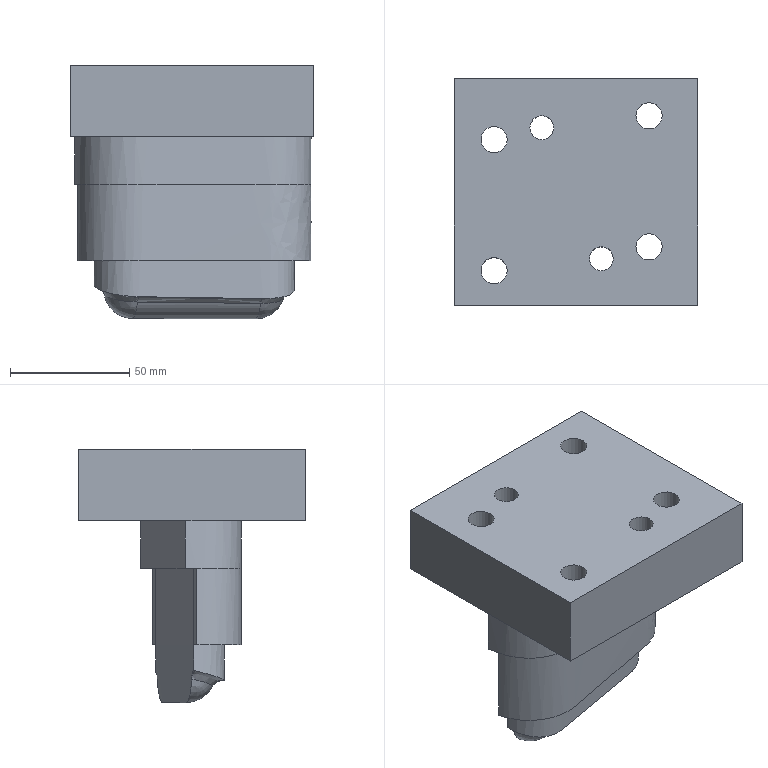Part | NX | features solid 2 | 1 solid | 39 faces | box 102 x 95 x 106.359 mm | volume 411302 mm3 | spline 17 | plane 12 | cylinder 10 | commonest cylinder face diameters 11 x4 17 x4 10 x2